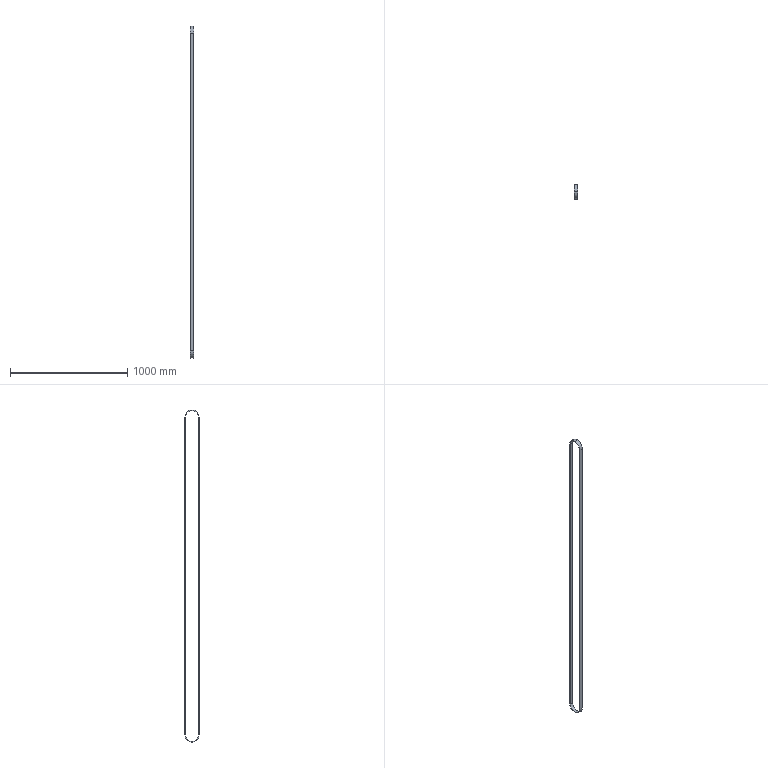Part | SolidWorks | features ExtruThin 1 | 1 solid | 12 faces | box 30 x 121.59 x 2832 mm | volume 781360 mm3 | cylinder 6 | plane 6 | commonest cylinder face diameters 112.59 x3 121.59 x3
STEP:
#1=CARTESIAN_POINT('',(15.,56.295,2710.));
#2=VERTEX_POINT('',#1);
#3=CARTESIAN_POINT('',(15.,0.,2766.295));
#4=VERTEX_POINT('',#3);
#5=CARTESIAN_POINT('',(15.,0.,2710.));
#6=DIRECTION('',(1.,0.,0.));
#7=DIRECTION('',(0.,0.,-1.));
#8=AXIS2_PLACEMENT_3D('',#5,#6,#7);
#9=CIRCLE('',#8,56.295);
#10=EDGE_CURVE('',#2,#4,#9,.T.);
#11=ORIENTED_EDGE('',*,*,#10,.T.);
#12=CARTESIAN_POINT('',(-15.,0.,2766.295));
#13=VERTEX_POINT('',#12);
#14=CARTESIAN_POINT('',(15.,0.,2766.295));
#15=DIRECTION('',(-1.,0.,0.));
#16=VECTOR('',#15,1000.);
#17=LINE('',#14,#16);
#18=EDGE_CURVE('',#4,#13,#17,.T.);
#19=ORIENTED_EDGE('',*,*,#18,.T.);
#20=CARTESIAN_POINT('',(-15.,56.295,2710.));
#21=VERTEX_POINT('',#20);
#22=CARTESIAN_POINT('',(-15.,0.,2710.));
#23=DIRECTION('',(1.,0.,0.));
#24=DIRECTION('',(0.,0.,-1.));
#25=AXIS2_PLACEMENT_3D('',#22,#23,#24);
#26=CIRCLE('',#25,56.295);
#27=EDGE_CURVE('',#21,#13,#26,.T.);
#28=ORIENTED_EDGE('',*,*,#27,.F.);
#29=CARTESIAN_POINT('',(15.,56.295,2710.));
#30=DIRECTION('',(-1.,0.,0.));
#31=VECTOR('',#30,1000.);
#32=LINE('',#29,#31);
#33=EDGE_CURVE('',#2,#21,#32,.T.);
#34=ORIENTED_EDGE('',*,*,#33,.F.);
#35=EDGE_LOOP('',(#11,#19,#28,#34));
#36=FACE_OUTER_BOUND('',#35,.T.);
#37=CARTESIAN_POINT('',(15.,0.,2710.));
#38=DIRECTION('',(-1.,0.,0.));
#39=DIRECTION('',(0.,0.,1.));
#40=AXIS2_PLACEMENT_3D('',#37,#38,#39);
#41=CYLINDRICAL_SURFACE('',#40,56.295);
#42=ADVANCED_FACE('',(#36),#41,.F.);
#43=CARTESIAN_POINT('',(15.,0.,2770.795));
#44=VERTEX_POINT('',#43);
#45=CARTESIAN_POINT('',(15.,-60.795,2710.));
#46=VERTEX_POINT('',#45);
#47=CARTESIAN_POINT('',(15.,0.,2710.));
#48=DIRECTION('',(1.,0.,0.));
#49=DIRECTION('',(0.,0.,-1.));
#50=AXIS2_PLACEMENT_3D('',#47,#48,#49);
#51=CIRCLE('',#50,60.795);
#52=EDGE_CURVE('',#44,#46,#51,.T.);
#53=ORIENTED_EDGE('',*,*,#52,.F.);
#54=CARTESIAN_POINT('',(-15.,0.,2770.795));
#55=VERTEX_POINT('',#54);
#56=CARTESIAN_POINT('',(15.,0.,2770.795));
#57=DIRECTION('',(-1.,0.,0.));
#58=VECTOR('',#57,1000.);
#59=LINE('',#56,#58);
#60=EDGE_CURVE('',#44,#55,#59,.T.);
#61=ORIENTED_EDGE('',*,*,#60,.T.);
#62=CARTESIAN_POINT('',(-15.,-60.795,2710.));
#63=VERTEX_POINT('',#62);
#64=CARTESIAN_POINT('',(-15.,0.,2710.));
#65=DIRECTION('',(1.,0.,0.));
#66=DIRECTION('',(0.,0.,-1.));
#67=AXIS2_PLACEMENT_3D('',#64,#65,#66);
#68=CIRCLE('',#67,60.795);
#69=EDGE_CURVE('',#55,#63,#68,.T.);
#70=ORIENTED_EDGE('',*,*,#69,.T.);
#71=CARTESIAN_POINT('',(15.,-60.795,2710.));
#72=DIRECTION('',(-1.,0.,0.));
#73=VECTOR('',#72,1000.);
#74=LINE('',#71,#73);
#75=EDGE_CURVE('',#46,#63,#74,.T.);
#76=ORIENTED_EDGE('',*,*,#75,.F.);
#77=EDGE_LOOP('',(#53,#61,#70,#76));
#78=FACE_OUTER_BOUND('',#77,.T.);
#79=CARTESIAN_POINT('',(15.,0.,2710.));
#80=DIRECTION('',(-1.,0.,0.));
#81=DIRECTION('',(0.,0.,1.));
#82=AXIS2_PLACEMENT_3D('',#79,#80,#81);
#83=CYLINDRICAL_SURFACE('',#82,60.795);
#84=ADVANCED_FACE('',(#78),#83,.T.);
#85=CARTESIAN_POINT('',(15.,60.795,2710.));
#86=VERTEX_POINT('',#85);
#87=CARTESIAN_POINT('',(15.,0.,2710.));
#88=DIRECTION('',(1.,0.,0.));
#89=DIRECTION('',(0.,0.,-1.));
#90=AXIS2_PLACEMENT_3D('',#87,#88,#89);
#91=CIRCLE('',#90,60.795);
#92=EDGE_CURVE('',#86,#44,#91,.T.);
#93=ORIENTED_EDGE('',*,*,#92,.T.);
#94=ORIENTED_EDGE('',*,*,#52,.T.);
#95=CARTESIAN_POINT('',(15.,-60.795,0.));
#96=VERTEX_POINT('',#95);
#97=CARTESIAN_POINT('',(15.,-60.795,2710.));
#98=DIRECTION('',(0.,0.,-1.));
#99=VECTOR('',#98,1000.);
#100=LINE('',#97,#99);
#101=EDGE_CURVE('',#46,#96,#100,.T.);
#102=ORIENTED_EDGE('',*,*,#101,.T.);
#103=CARTESIAN_POINT('',(15.,60.795,0.));
#104=VERTEX_POINT('',#103);
#105=CARTESIAN_POINT('',(15.,0.,0.));
#106=DIRECTION('',(1.,0.,0.));
#107=DIRECTION('',(0.,0.,-1.));
#108=AXIS2_PLACEMENT_3D('',#105,#106,#107);
#109=CIRCLE('',#108,60.795);
#110=EDGE_CURVE('',#96,#104,#109,.T.);
#111=ORIENTED_EDGE('',*,*,#110,.T.);
#112=CARTESIAN_POINT('',(15.,60.795,0.));
#113=DIRECTION('',(0.,0.,1.));
#114=VECTOR('',#113,1000.);
#115=LINE('',#112,#114);
#116=EDGE_CURVE('',#104,#86,#115,.T.);
#117=ORIENTED_EDGE('',*,*,#116,.T.);
#118=EDGE_LOOP('',(#93,#94,#102,#111,#117));
#119=FACE_OUTER_BOUND('',#118,.T.);
#120=CARTESIAN_POINT('',(15.,-56.295,2710.));
#121=VERTEX_POINT('',#120);
#122=CARTESIAN_POINT('',(15.,-56.295,0.));
#123=VERTEX_POINT('',#122);
#124=CARTESIAN_POINT('',(15.,-56.295,2710.));
#125=DIRECTION('',(0.,0.,-1.));
#126=VECTOR('',#125,1000.);
#127=LINE('',#124,#126);
#128=EDGE_CURVE('',#121,#123,#127,.T.);
#129=ORIENTED_EDGE('',*,*,#128,.F.);
#130=CARTESIAN_POINT('',(15.,0.,2710.));
#131=DIRECTION('',(1.,0.,0.));
#132=DIRECTION('',(0.,0.,-1.));
#133=AXIS2_PLACEMENT_3D('',#130,#131,#132);
#134=CIRCLE('',#133,56.295);
#135=EDGE_CURVE('',#4,#121,#134,.T.);
#136=ORIENTED_EDGE('',*,*,#135,.F.);
#137=ORIENTED_EDGE('',*,*,#10,.F.);
#138=CARTESIAN_POINT('',(15.,56.295,0.));
#139=VERTEX_POINT('',#138);
#140=CARTESIAN_POINT('',(15.,56.295,0.));
#141=DIRECTION('',(0.,0.,1.));
#142=VECTOR('',#141,1000.);
#143=LINE('',#140,#142);
#144=EDGE_CURVE('',#139,#2,#143,.T.);
#145=ORIENTED_EDGE('',*,*,#144,.F.);
#146=CARTESIAN_POINT('',(15.,0.,0.));
#147=DIRECTION('',(1.,0.,0.));
#148=DIRECTION('',(0.,0.,-1.));
#149=AXIS2_PLACEMENT_3D('',#146,#147,#148);
#150=CIRCLE('',#149,56.295);
#151=EDGE_CURVE('',#123,#139,#150,.T.);
#152=ORIENTED_EDGE('',*,*,#151,.F.);
#153=EDGE_LOOP('',(#129,#136,#137,#145,#152));
#154=FACE_BOUND('',#153,.T.);
#155=CARTESIAN_POINT('',(15.,0.,2710.));
#156=DIRECTION('',(1.,0.,0.));
#157=DIRECTION('',(0.,0.,-1.));
#158=AXIS2_PLACEMENT_3D('',#155,#156,#157);
#159=PLANE('',#158);
#160=ADVANCED_FACE('',(#119,#154),#159,.T.);
#161=CARTESIAN_POINT('',(-15.,60.795,2710.));
#162=VERTEX_POINT('',#161);
#163=CARTESIAN_POINT('',(-15.,0.,2710.));
#164=DIRECTION('',(1.,0.,0.));
#165=DIRECTION('',(0.,0.,-1.));
#166=AXIS2_PLACEMENT_3D('',#163,#164,#165);
#167=CIRCLE('',#166,60.795);
#168=EDGE_CURVE('',#162,#55,#167,.T.);
#169=ORIENTED_EDGE('',*,*,#168,.F.);
#170=CARTESIAN_POINT('',(-15.,60.795,0.));
#171=VERTEX_POINT('',#170);
#172=CARTESIAN_POINT('',(-15.,60.795,0.));
#173=DIRECTION('',(0.,0.,1.));
#174=VECTOR('',#173,1000.);
#175=LINE('',#172,#174);
#176=EDGE_CURVE('',#171,#162,#175,.T.);
#177=ORIENTED_EDGE('',*,*,#176,.F.);
#178=CARTESIAN_POINT('',(-15.,-60.795,0.));
#179=VERTEX_POINT('',#178);
#180=CARTESIAN_POINT('',(-15.,0.,0.));
#181=DIRECTION('',(1.,0.,0.));
#182=DIRECTION('',(0.,0.,-1.));
#183=AXIS2_PLACEMENT_3D('',#180,#181,#182);
#184=CIRCLE('',#183,60.795);
#185=EDGE_CURVE('',#179,#171,#184,.T.);
#186=ORIENTED_EDGE('',*,*,#185,.F.);
#187=CARTESIAN_POINT('',(-15.,-60.795,2710.));
#188=DIRECTION('',(0.,0.,-1.));
#189=VECTOR('',#188,1000.);
#190=LINE('',#187,#189);
#191=EDGE_CURVE('',#63,#179,#190,.T.);
#192=ORIENTED_EDGE('',*,*,#191,.F.);
#193=ORIENTED_EDGE('',*,*,#69,.F.);
#194=EDGE_LOOP('',(#169,#177,#186,#192,#193));
#195=FACE_OUTER_BOUND('',#194,.T.);
#196=ORIENTED_EDGE('',*,*,#27,.T.);
#197=CARTESIAN_POINT('',(-15.,-56.295,2710.));
#198=VERTEX_POINT('',#197);
#199=CARTESIAN_POINT('',(-15.,0.,2710.));
#200=DIRECTION('',(1.,0.,0.));
#201=DIRECTION('',(0.,0.,-1.));
#202=AXIS2_PLACEMENT_3D('',#199,#200,#201);
#203=CIRCLE('',#202,56.295);
#204=EDGE_CURVE('',#13,#198,#203,.T.);
#205=ORIENTED_EDGE('',*,*,#204,.T.);
#206=CARTESIAN_POINT('',(-15.,-56.295,0.));
#207=VERTEX_POINT('',#206);
#208=CARTESIAN_POINT('',(-15.,-56.295,2710.));
#209=DIRECTION('',(0.,0.,-1.));
#210=VECTOR('',#209,1000.);
#211=LINE('',#208,#210);
#212=EDGE_CURVE('',#198,#207,#211,.T.);
#213=ORIENTED_EDGE('',*,*,#212,.T.);
#214=CARTESIAN_POINT('',(-15.,56.295,0.));
#215=VERTEX_POINT('',#214);
#216=CARTESIAN_POINT('',(-15.,0.,0.));
#217=DIRECTION('',(1.,0.,0.));
#218=DIRECTION('',(0.,0.,-1.));
#219=AXIS2_PLACEMENT_3D('',#216,#217,#218);
#220=CIRCLE('',#219,56.295);
#221=EDGE_CURVE('',#207,#215,#220,.T.);
#222=ORIENTED_EDGE('',*,*,#221,.T.);
#223=CARTESIAN_POINT('',(-15.,56.295,0.));
#224=DIRECTION('',(0.,0.,1.));
#225=VECTOR('',#224,1000.);
#226=LINE('',#223,#225);
#227=EDGE_CURVE('',#215,#21,#226,.T.);
#228=ORIENTED_EDGE('',*,*,#227,.T.);
#229=EDGE_LOOP('',(#196,#205,#213,#222,#228));
#230=FACE_BOUND('',#229,.T.);
#231=CARTESIAN_POINT('',(-15.,0.,2710.));
#232=DIRECTION('',(1.,0.,0.));
#233=DIRECTION('',(0.,0.,-1.));
#234=AXIS2_PLACEMENT_3D('',#231,#232,#233);
#235=PLANE('',#234);
#236=ADVANCED_FACE('',(#195,#230),#235,.F.);
#237=ORIENTED_EDGE('',*,*,#60,.F.);
#238=ORIENTED_EDGE('',*,*,#92,.F.);
#239=CARTESIAN_POINT('',(15.,60.795,2710.));
#240=DIRECTION('',(-1.,0.,0.));
#241=VECTOR('',#240,1000.);
#242=LINE('',#239,#241);
#243=EDGE_CURVE('',#86,#162,#242,.T.);
#244=ORIENTED_EDGE('',*,*,#243,.T.);
#245=ORIENTED_EDGE('',*,*,#168,.T.);
#246=EDGE_LOOP('',(#237,#238,#244,#245));
#247=FACE_OUTER_BOUND('',#246,.T.);
#248=CARTESIAN_POINT('',(15.,0.,2710.));
#249=DIRECTION('',(-1.,0.,0.));
#250=DIRECTION('',(0.,0.,1.));
#251=AXIS2_PLACEMENT_3D('',#248,#249,#250);
#252=CYLINDRICAL_SURFACE('',#251,60.795);
#253=ADVANCED_FACE('',(#247),#252,.T.);
#254=ORIENTED_EDGE('',*,*,#191,.T.);
#255=CARTESIAN_POINT('',(15.,-60.795,0.));
#256=DIRECTION('',(-1.,0.,0.));
#257=VECTOR('',#256,1000.);
#258=LINE('',#255,#257);
#259=EDGE_CURVE('',#96,#179,#258,.T.);
#260=ORIENTED_EDGE('',*,*,#259,.F.);
#261=ORIENTED_EDGE('',*,*,#101,.F.);
#262=ORIENTED_EDGE('',*,*,#75,.T.);
#263=EDGE_LOOP('',(#254,#260,#261,#262));
#264=FACE_OUTER_BOUND('',#263,.T.);
#265=CARTESIAN_POINT('',(15.,-60.795,2710.));
#266=DIRECTION('',(0.,1.,0.));
#267=DIRECTION('',(0.,0.,1.));
#268=AXIS2_PLACEMENT_3D('',#265,#266,#267);
#269=PLANE('',#268);
#270=ADVANCED_FACE('',(#264),#269,.F.);
#271=ORIENTED_EDGE('',*,*,#185,.T.);
#272=CARTESIAN_POINT('',(15.,60.795,0.));
#273=DIRECTION('',(-1.,0.,0.));
#274=VECTOR('',#273,1000.);
#275=LINE('',#272,#274);
#276=EDGE_CURVE('',#104,#171,#275,.T.);
#277=ORIENTED_EDGE('',*,*,#276,.F.);
#278=ORIENTED_EDGE('',*,*,#110,.F.);
#279=ORIENTED_EDGE('',*,*,#259,.T.);
#280=EDGE_LOOP('',(#271,#277,#278,#279));
#281=FACE_OUTER_BOUND('',#280,.T.);
#282=CARTESIAN_POINT('',(15.,0.,0.));
#283=DIRECTION('',(-1.,0.,0.));
#284=DIRECTION('',(0.,0.,1.));
#285=AXIS2_PLACEMENT_3D('',#282,#283,#284);
#286=CYLINDRICAL_SURFACE('',#285,60.795);
#287=ADVANCED_FACE('',(#281),#286,.T.);
#288=ORIENTED_EDGE('',*,*,#176,.T.);
#289=ORIENTED_EDGE('',*,*,#243,.F.);
#290=ORIENTED_EDGE('',*,*,#116,.F.);
#291=ORIENTED_EDGE('',*,*,#276,.T.);
#292=EDGE_LOOP('',(#288,#289,#290,#291));
#293=FACE_OUTER_BOUND('',#292,.T.);
#294=CARTESIAN_POINT('',(15.,60.795,0.));
#295=DIRECTION('',(0.,-1.,0.));
#296=DIRECTION('',(0.,0.,-1.));
#297=AXIS2_PLACEMENT_3D('',#294,#295,#296);
#298=PLANE('',#297);
#299=ADVANCED_FACE('',(#293),#298,.F.);
#300=ORIENTED_EDGE('',*,*,#18,.F.);
#301=ORIENTED_EDGE('',*,*,#135,.T.);
#302=CARTESIAN_POINT('',(15.,-56.295,2710.));
#303=DIRECTION('',(-1.,0.,0.));
#304=VECTOR('',#303,1000.);
#305=LINE('',#302,#304);
#306=EDGE_CURVE('',#121,#198,#305,.T.);
#307=ORIENTED_EDGE('',*,*,#306,.T.);
#308=ORIENTED_EDGE('',*,*,#204,.F.);
#309=EDGE_LOOP('',(#300,#301,#307,#308));
#310=FACE_OUTER_BOUND('',#309,.T.);
#311=CARTESIAN_POINT('',(15.,0.,2710.));
#312=DIRECTION('',(-1.,0.,0.));
#313=DIRECTION('',(0.,0.,1.));
#314=AXIS2_PLACEMENT_3D('',#311,#312,#313);
#315=CYLINDRICAL_SURFACE('',#314,56.295);
#316=ADVANCED_FACE('',(#310),#315,.F.);
#317=ORIENTED_EDGE('',*,*,#212,.F.);
#318=ORIENTED_EDGE('',*,*,#306,.F.);
#319=ORIENTED_EDGE('',*,*,#128,.T.);
#320=CARTESIAN_POINT('',(15.,-56.295,0.));
#321=DIRECTION('',(-1.,0.,0.));
#322=VECTOR('',#321,1000.);
#323=LINE('',#320,#322);
#324=EDGE_CURVE('',#123,#207,#323,.T.);
#325=ORIENTED_EDGE('',*,*,#324,.T.);
#326=EDGE_LOOP('',(#317,#318,#319,#325));
#327=FACE_OUTER_BOUND('',#326,.T.);
#328=CARTESIAN_POINT('',(15.,-56.295,2710.));
#329=DIRECTION('',(0.,1.,0.));
#330=DIRECTION('',(0.,0.,1.));
#331=AXIS2_PLACEMENT_3D('',#328,#329,#330);
#332=PLANE('',#331);
#333=ADVANCED_FACE('',(#327),#332,.T.);
#334=ORIENTED_EDGE('',*,*,#221,.F.);
#335=ORIENTED_EDGE('',*,*,#324,.F.);
#336=ORIENTED_EDGE('',*,*,#151,.T.);
#337=CARTESIAN_POINT('',(15.,56.295,0.));
#338=DIRECTION('',(-1.,0.,0.));
#339=VECTOR('',#338,1000.);
#340=LINE('',#337,#339);
#341=EDGE_CURVE('',#139,#215,#340,.T.);
#342=ORIENTED_EDGE('',*,*,#341,.T.);
#343=EDGE_LOOP('',(#334,#335,#336,#342));
#344=FACE_OUTER_BOUND('',#343,.T.);
#345=CARTESIAN_POINT('',(15.,0.,0.));
#346=DIRECTION('',(-1.,0.,0.));
#347=DIRECTION('',(0.,0.,1.));
#348=AXIS2_PLACEMENT_3D('',#345,#346,#347);
#349=CYLINDRICAL_SURFACE('',#348,56.295);
#350=ADVANCED_FACE('',(#344),#349,.F.);
#351=ORIENTED_EDGE('',*,*,#227,.F.);
#352=ORIENTED_EDGE('',*,*,#341,.F.);
#353=ORIENTED_EDGE('',*,*,#144,.T.);
#354=ORIENTED_EDGE('',*,*,#33,.T.);
#355=EDGE_LOOP('',(#351,#352,#353,#354));
#356=FACE_OUTER_BOUND('',#355,.T.);
#357=CARTESIAN_POINT('',(15.,56.295,0.));
#358=DIRECTION('',(0.,-1.,0.));
#359=DIRECTION('',(0.,0.,-1.));
#360=AXIS2_PLACEMENT_3D('',#357,#358,#359);
#361=PLANE('',#360);
#362=ADVANCED_FACE('',(#356),#361,.T.);
#363=CLOSED_SHELL('',(#42,#84,#160,#236,#253,#270,#287,#299,#316,#333,#350,#362));
#364=MANIFOLD_SOLID_BREP('',#363);
#365=CARTESIAN_POINT('',(0.,0.,0.));
#366=DIRECTION('',(0.,0.,1.));
#367=DIRECTION('',(1.,0.,0.));
#368=AXIS2_PLACEMENT_3D('',#365,#366,#367);
#369=(LENGTH_UNIT()NAMED_UNIT(*)SI_UNIT(.MILLI.,.METRE.));
#370=UNCERTAINTY_MEASURE_WITH_UNIT(LENGTH_MEASURE(0.00001),#369,'','');
#371=(NAMED_UNIT(*)PLANE_ANGLE_UNIT()SI_UNIT($,.RADIAN.));
#372=(NAMED_UNIT(*)SI_UNIT($,.STERADIAN.)SOLID_ANGLE_UNIT());
#373=(GEOMETRIC_REPRESENTATION_CONTEXT(3)GLOBAL_UNCERTAINTY_ASSIGNED_CONTEXT((#370))GLOBAL_UNIT_ASSIGNED_CONTEXT((#369,#371,#372))REPRESENTATION_CONTEXT('',''));
#374=ADVANCED_BREP_SHAPE_REPRESENTATION('',(#364,#368),#373);